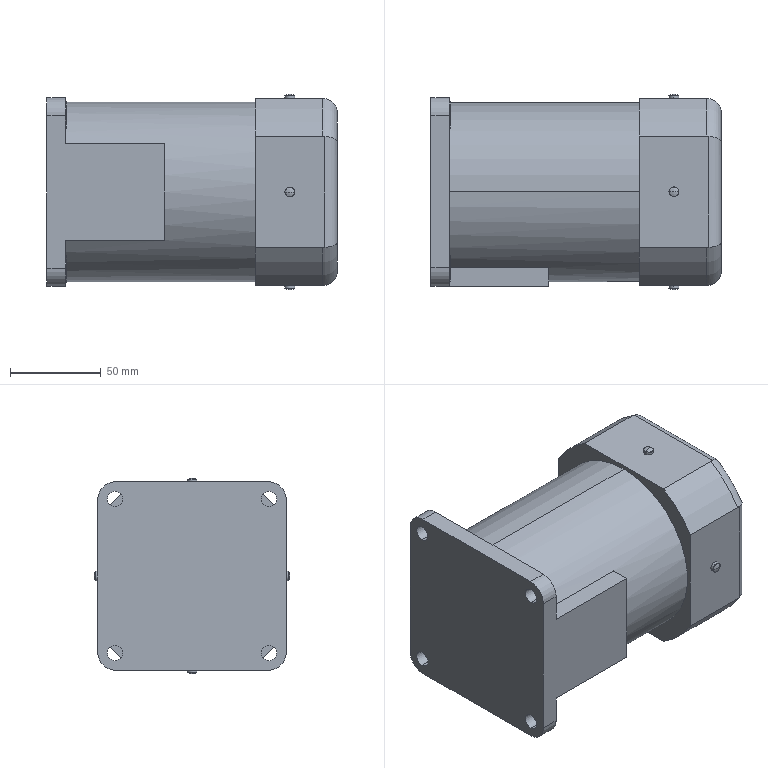Part | STEP file | OM-BHI62E-5RA-CC05AC33P-EPCR1201-2_200W_A_Motor-1 | 1 solid | 152 faces | box 160 x 107.8 x 107.8 mm | volume 1356230 mm3 | cylinder 100 | plane 32 | torus 12 | sphere 8 | commonest cylinder face diameters 5 x36 5.5 x8 8.5 x8 14.5 x8 16 x4 20 x4